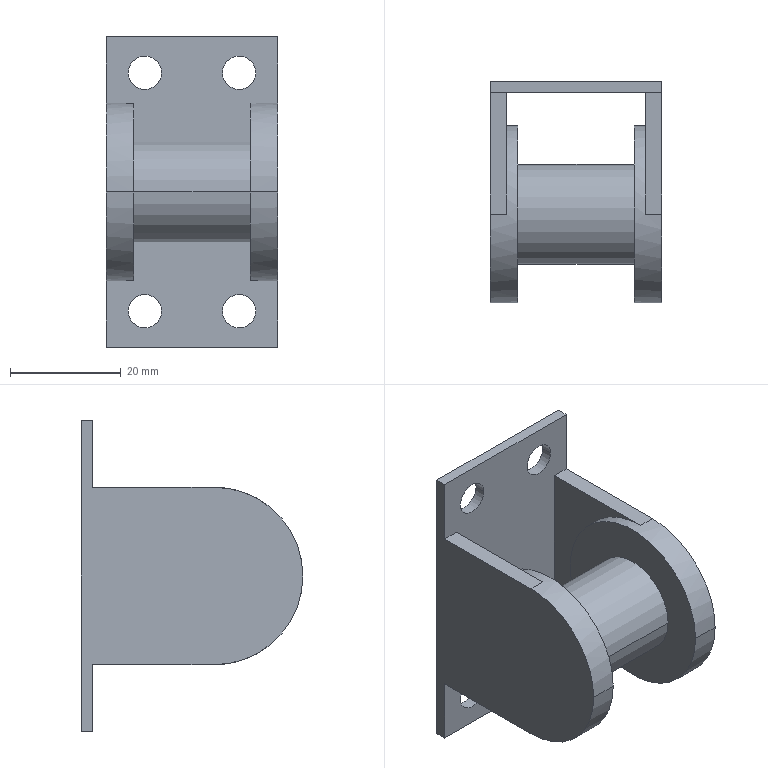Part | SolidWorks | features ICE 3, MirrorPattern 1, Revolution 1 | 1 solid | 28 faces | box 31 x 40 x 56 mm | volume 18443 mm3 | cylinder 14 | plane 14 | commonest cylinder face diameters 6 x8 32 x4 18 x2
STEP:
#1=CARTESIAN_POINT('',(18.,22.,-21.5));
#2=VERTEX_POINT('',#1);
#3=CARTESIAN_POINT('',(24.,22.,-21.5));
#4=VERTEX_POINT('',#3);
#5=CARTESIAN_POINT('',(21.,22.,-21.5));
#6=DIRECTION('',(0.,-1.,0.));
#7=DIRECTION('',(0.,0.,1.));
#8=AXIS2_PLACEMENT_3D('',#5,#6,#7);
#9=CIRCLE('',#8,3.);
#10=EDGE_CURVE('',#2,#4,#9,.T.);
#11=ORIENTED_EDGE('',*,*,#10,.T.);
#12=CARTESIAN_POINT('',(24.,24.,-21.5));
#13=VERTEX_POINT('',#12);
#14=CARTESIAN_POINT('',(24.,-16.001,-21.5));
#15=DIRECTION('',(0.,1.,0.));
#16=VECTOR('',#15,1000.);
#17=LINE('',#14,#16);
#18=EDGE_CURVE('',#4,#13,#17,.T.);
#19=ORIENTED_EDGE('',*,*,#18,.T.);
#20=CARTESIAN_POINT('',(18.,24.,-21.5));
#21=VERTEX_POINT('',#20);
#22=CARTESIAN_POINT('',(21.,24.,-21.5));
#23=DIRECTION('',(0.,1.,0.));
#24=DIRECTION('',(1.,0.,0.));
#25=AXIS2_PLACEMENT_3D('',#22,#23,#24);
#26=CIRCLE('',#25,3.);
#27=EDGE_CURVE('',#13,#21,#26,.T.);
#28=ORIENTED_EDGE('',*,*,#27,.T.);
#29=CARTESIAN_POINT('',(18.,-16.001,-21.5));
#30=DIRECTION('',(0.,1.,0.));
#31=VECTOR('',#30,1000.);
#32=LINE('',#29,#31);
#33=EDGE_CURVE('',#2,#21,#32,.T.);
#34=ORIENTED_EDGE('',*,*,#33,.F.);
#35=EDGE_LOOP('',(#11,#19,#28,#34));
#36=FACE_OUTER_BOUND('',#35,.T.);
#37=CARTESIAN_POINT('',(21.,-16.001,-21.5));
#38=DIRECTION('',(0.,1.,0.));
#39=DIRECTION('',(-1.,0.,0.));
#40=AXIS2_PLACEMENT_3D('',#37,#38,#39);
#41=CYLINDRICAL_SURFACE('',#40,3.);
#42=ADVANCED_FACE('',(#36),#41,.F.);
#43=CARTESIAN_POINT('',(18.,22.,21.5));
#44=VERTEX_POINT('',#43);
#45=CARTESIAN_POINT('',(24.,22.,21.5));
#46=VERTEX_POINT('',#45);
#47=CARTESIAN_POINT('',(21.,22.,21.5));
#48=DIRECTION('',(0.,-1.,0.));
#49=DIRECTION('',(0.,0.,1.));
#50=AXIS2_PLACEMENT_3D('',#47,#48,#49);
#51=CIRCLE('',#50,3.);
#52=EDGE_CURVE('',#44,#46,#51,.T.);
#53=ORIENTED_EDGE('',*,*,#52,.T.);
#54=CARTESIAN_POINT('',(24.,24.,21.5));
#55=VERTEX_POINT('',#54);
#56=CARTESIAN_POINT('',(24.,-16.001,21.5));
#57=DIRECTION('',(0.,1.,0.));
#58=VECTOR('',#57,1000.);
#59=LINE('',#56,#58);
#60=EDGE_CURVE('',#46,#55,#59,.T.);
#61=ORIENTED_EDGE('',*,*,#60,.T.);
#62=CARTESIAN_POINT('',(18.,24.,21.5));
#63=VERTEX_POINT('',#62);
#64=CARTESIAN_POINT('',(21.,24.,21.5));
#65=DIRECTION('',(0.,1.,0.));
#66=DIRECTION('',(-1.,0.,0.));
#67=AXIS2_PLACEMENT_3D('',#64,#65,#66);
#68=CIRCLE('',#67,3.);
#69=EDGE_CURVE('',#55,#63,#68,.T.);
#70=ORIENTED_EDGE('',*,*,#69,.T.);
#71=CARTESIAN_POINT('',(18.,-16.001,21.5));
#72=DIRECTION('',(0.,1.,0.));
#73=VECTOR('',#72,1000.);
#74=LINE('',#71,#73);
#75=EDGE_CURVE('',#44,#63,#74,.T.);
#76=ORIENTED_EDGE('',*,*,#75,.F.);
#77=EDGE_LOOP('',(#53,#61,#70,#76));
#78=FACE_OUTER_BOUND('',#77,.T.);
#79=CARTESIAN_POINT('',(21.,-16.001,21.5));
#80=DIRECTION('',(0.,1.,0.));
#81=DIRECTION('',(-1.,0.,0.));
#82=AXIS2_PLACEMENT_3D('',#79,#80,#81);
#83=CYLINDRICAL_SURFACE('',#82,3.);
#84=ADVANCED_FACE('',(#78),#83,.F.);
#85=CARTESIAN_POINT('',(1.,22.,21.5));
#86=VERTEX_POINT('',#85);
#87=CARTESIAN_POINT('',(7.,22.,21.5));
#88=VERTEX_POINT('',#87);
#89=CARTESIAN_POINT('',(4.,22.,21.5));
#90=DIRECTION('',(0.,-1.,0.));
#91=DIRECTION('',(0.,0.,1.));
#92=AXIS2_PLACEMENT_3D('',#89,#90,#91);
#93=CIRCLE('',#92,3.);
#94=EDGE_CURVE('',#86,#88,#93,.T.);
#95=ORIENTED_EDGE('',*,*,#94,.T.);
#96=CARTESIAN_POINT('',(7.,24.,21.5));
#97=VERTEX_POINT('',#96);
#98=CARTESIAN_POINT('',(7.,-16.001,21.5));
#99=DIRECTION('',(0.,1.,0.));
#100=VECTOR('',#99,1000.);
#101=LINE('',#98,#100);
#102=EDGE_CURVE('',#88,#97,#101,.T.);
#103=ORIENTED_EDGE('',*,*,#102,.T.);
#104=CARTESIAN_POINT('',(1.,24.,21.5));
#105=VERTEX_POINT('',#104);
#106=CARTESIAN_POINT('',(4.,24.,21.5));
#107=DIRECTION('',(0.,1.,0.));
#108=DIRECTION('',(1.,0.,0.));
#109=AXIS2_PLACEMENT_3D('',#106,#107,#108);
#110=CIRCLE('',#109,3.);
#111=EDGE_CURVE('',#97,#105,#110,.T.);
#112=ORIENTED_EDGE('',*,*,#111,.T.);
#113=CARTESIAN_POINT('',(1.,-16.001,21.5));
#114=DIRECTION('',(0.,1.,0.));
#115=VECTOR('',#114,1000.);
#116=LINE('',#113,#115);
#117=EDGE_CURVE('',#86,#105,#116,.T.);
#118=ORIENTED_EDGE('',*,*,#117,.F.);
#119=EDGE_LOOP('',(#95,#103,#112,#118));
#120=FACE_OUTER_BOUND('',#119,.T.);
#121=CARTESIAN_POINT('',(4.,-16.001,21.5));
#122=DIRECTION('',(0.,1.,0.));
#123=DIRECTION('',(-1.,0.,0.));
#124=AXIS2_PLACEMENT_3D('',#121,#122,#123);
#125=CYLINDRICAL_SURFACE('',#124,3.);
#126=ADVANCED_FACE('',(#120),#125,.F.);
#127=CARTESIAN_POINT('',(1.,22.,-21.5));
#128=VERTEX_POINT('',#127);
#129=CARTESIAN_POINT('',(7.,22.,-21.5));
#130=VERTEX_POINT('',#129);
#131=CARTESIAN_POINT('',(4.,22.,-21.5));
#132=DIRECTION('',(0.,-1.,0.));
#133=DIRECTION('',(0.,0.,1.));
#134=AXIS2_PLACEMENT_3D('',#131,#132,#133);
#135=CIRCLE('',#134,3.);
#136=EDGE_CURVE('',#128,#130,#135,.T.);
#137=ORIENTED_EDGE('',*,*,#136,.T.);
#138=CARTESIAN_POINT('',(7.,24.,-21.5));
#139=VERTEX_POINT('',#138);
#140=CARTESIAN_POINT('',(7.,-16.001,-21.5));
#141=DIRECTION('',(0.,1.,0.));
#142=VECTOR('',#141,1000.);
#143=LINE('',#140,#142);
#144=EDGE_CURVE('',#130,#139,#143,.T.);
#145=ORIENTED_EDGE('',*,*,#144,.T.);
#146=CARTESIAN_POINT('',(1.,24.,-21.5));
#147=VERTEX_POINT('',#146);
#148=CARTESIAN_POINT('',(4.,24.,-21.5));
#149=DIRECTION('',(0.,1.,0.));
#150=DIRECTION('',(-1.,0.,0.));
#151=AXIS2_PLACEMENT_3D('',#148,#149,#150);
#152=CIRCLE('',#151,3.);
#153=EDGE_CURVE('',#139,#147,#152,.T.);
#154=ORIENTED_EDGE('',*,*,#153,.T.);
#155=CARTESIAN_POINT('',(1.,-16.001,-21.5));
#156=DIRECTION('',(0.,1.,0.));
#157=VECTOR('',#156,1000.);
#158=LINE('',#155,#157);
#159=EDGE_CURVE('',#128,#147,#158,.T.);
#160=ORIENTED_EDGE('',*,*,#159,.F.);
#161=EDGE_LOOP('',(#137,#145,#154,#160));
#162=FACE_OUTER_BOUND('',#161,.T.);
#163=CARTESIAN_POINT('',(4.,-16.001,-21.5));
#164=DIRECTION('',(0.,1.,0.));
#165=DIRECTION('',(-1.,0.,0.));
#166=AXIS2_PLACEMENT_3D('',#163,#164,#165);
#167=CYLINDRICAL_SURFACE('',#166,3.);
#168=ADVANCED_FACE('',(#162),#167,.F.);
#169=CARTESIAN_POINT('',(2.,9.,0.));
#170=VERTEX_POINT('',#169);
#171=CARTESIAN_POINT('',(2.,-9.,0.));
#172=VERTEX_POINT('',#171);
#173=CARTESIAN_POINT('',(2.,0.,0.));
#174=DIRECTION('',(1.,0.,0.));
#175=DIRECTION('',(0.,1.,0.));
#176=AXIS2_PLACEMENT_3D('',#173,#174,#175);
#177=CIRCLE('',#176,9.);
#178=EDGE_CURVE('',#170,#172,#177,.T.);
#179=ORIENTED_EDGE('',*,*,#178,.T.);
#180=CARTESIAN_POINT('',(23.,-9.,0.));
#181=VERTEX_POINT('',#180);
#182=CARTESIAN_POINT('',(25.,-9.,0.));
#183=DIRECTION('',(1.,0.,0.));
#184=VECTOR('',#183,1000.);
#185=LINE('',#182,#184);
#186=EDGE_CURVE('',#172,#181,#185,.T.);
#187=ORIENTED_EDGE('',*,*,#186,.T.);
#188=CARTESIAN_POINT('',(23.,9.,0.));
#189=VERTEX_POINT('',#188);
#190=CARTESIAN_POINT('',(23.,0.,0.));
#191=DIRECTION('',(1.,0.,0.));
#192=DIRECTION('',(0.,1.,0.));
#193=AXIS2_PLACEMENT_3D('',#190,#191,#192);
#194=CIRCLE('',#193,9.);
#195=EDGE_CURVE('',#189,#181,#194,.T.);
#196=ORIENTED_EDGE('',*,*,#195,.F.);
#197=CARTESIAN_POINT('',(25.,9.,0.));
#198=DIRECTION('',(1.,0.,0.));
#199=VECTOR('',#198,1000.);
#200=LINE('',#197,#199);
#201=EDGE_CURVE('',#170,#189,#200,.T.);
#202=ORIENTED_EDGE('',*,*,#201,.F.);
#203=EDGE_LOOP('',(#179,#187,#196,#202));
#204=FACE_OUTER_BOUND('',#203,.T.);
#205=CARTESIAN_POINT('',(25.,0.,0.));
#206=DIRECTION('',(1.,0.,0.));
#207=DIRECTION('',(0.,1.,0.));
#208=AXIS2_PLACEMENT_3D('',#205,#206,#207);
#209=CYLINDRICAL_SURFACE('',#208,9.);
#210=ADVANCED_FACE('',(#204),#209,.T.);
#211=CARTESIAN_POINT('',(23.,16.,0.));
#212=VERTEX_POINT('',#211);
#213=CARTESIAN_POINT('',(23.,-16.,0.));
#214=VERTEX_POINT('',#213);
#215=CARTESIAN_POINT('',(23.,0.,0.));
#216=DIRECTION('',(1.,0.,0.));
#217=DIRECTION('',(0.,1.,0.));
#218=AXIS2_PLACEMENT_3D('',#215,#216,#217);
#219=CIRCLE('',#218,16.);
#220=EDGE_CURVE('',#212,#214,#219,.T.);
#221=ORIENTED_EDGE('',*,*,#220,.T.);
#222=CARTESIAN_POINT('',(28.,-16.,0.));
#223=VERTEX_POINT('',#222);
#224=CARTESIAN_POINT('',(25.,-16.,0.));
#225=DIRECTION('',(1.,0.,0.));
#226=VECTOR('',#225,1000.);
#227=LINE('',#224,#226);
#228=EDGE_CURVE('',#214,#223,#227,.T.);
#229=ORIENTED_EDGE('',*,*,#228,.T.);
#230=CARTESIAN_POINT('',(28.,0.,16.));
#231=VERTEX_POINT('',#230);
#232=CARTESIAN_POINT('',(28.,0.,0.));
#233=DIRECTION('',(-1.,0.,0.));
#234=DIRECTION('',(0.,-1.,0.));
#235=AXIS2_PLACEMENT_3D('',#232,#233,#234);
#236=CIRCLE('',#235,16.);
#237=EDGE_CURVE('',#223,#231,#236,.T.);
#238=ORIENTED_EDGE('',*,*,#237,.T.);
#239=CARTESIAN_POINT('',(25.,0.,16.));
#240=VERTEX_POINT('',#239);
#241=CARTESIAN_POINT('',(28.,0.,16.));
#242=DIRECTION('',(-1.,0.,0.));
#243=VECTOR('',#242,1000.);
#244=LINE('',#241,#243);
#245=EDGE_CURVE('',#231,#240,#244,.T.);
#246=ORIENTED_EDGE('',*,*,#245,.T.);
#247=CARTESIAN_POINT('',(25.,16.,0.));
#248=VERTEX_POINT('',#247);
#249=CARTESIAN_POINT('',(25.,0.,0.));
#250=DIRECTION('',(1.,0.,0.));
#251=DIRECTION('',(0.,1.,0.));
#252=AXIS2_PLACEMENT_3D('',#249,#250,#251);
#253=CIRCLE('',#252,16.);
#254=EDGE_CURVE('',#248,#240,#253,.T.);
#255=ORIENTED_EDGE('',*,*,#254,.F.);
#256=CARTESIAN_POINT('',(25.,16.,0.));
#257=DIRECTION('',(1.,0.,0.));
#258=VECTOR('',#257,1000.);
#259=LINE('',#256,#258);
#260=EDGE_CURVE('',#212,#248,#259,.T.);
#261=ORIENTED_EDGE('',*,*,#260,.F.);
#262=EDGE_LOOP('',(#221,#229,#238,#246,#255,#261));
#263=FACE_OUTER_BOUND('',#262,.T.);
#264=CARTESIAN_POINT('',(25.,0.,0.));
#265=DIRECTION('',(1.,0.,0.));
#266=DIRECTION('',(0.,1.,0.));
#267=AXIS2_PLACEMENT_3D('',#264,#265,#266);
#268=CYLINDRICAL_SURFACE('',#267,16.);
#269=ADVANCED_FACE('',(#263),#268,.T.);
#270=CARTESIAN_POINT('',(-3.,-16.,0.));
#271=VERTEX_POINT('',#270);
#272=CARTESIAN_POINT('',(-3.,0.,16.));
#273=VERTEX_POINT('',#272);
#274=CARTESIAN_POINT('',(-3.,0.,0.));
#275=DIRECTION('',(-1.,0.,0.));
#276=DIRECTION('',(0.,-1.,0.));
#277=AXIS2_PLACEMENT_3D('',#274,#275,#276);
#278=CIRCLE('',#277,16.);
#279=EDGE_CURVE('',#271,#273,#278,.T.);
#280=ORIENTED_EDGE('',*,*,#279,.F.);
#281=CARTESIAN_POINT('',(2.,-16.,0.));
#282=VERTEX_POINT('',#281);
#283=CARTESIAN_POINT('',(25.,-16.,0.));
#284=DIRECTION('',(1.,0.,0.));
#285=VECTOR('',#284,1000.);
#286=LINE('',#283,#285);
#287=EDGE_CURVE('',#271,#282,#286,.T.);
#288=ORIENTED_EDGE('',*,*,#287,.T.);
#289=CARTESIAN_POINT('',(2.,16.,0.));
#290=VERTEX_POINT('',#289);
#291=CARTESIAN_POINT('',(2.,0.,0.));
#292=DIRECTION('',(1.,0.,0.));
#293=DIRECTION('',(0.,1.,0.));
#294=AXIS2_PLACEMENT_3D('',#291,#292,#293);
#295=CIRCLE('',#294,16.);
#296=EDGE_CURVE('',#290,#282,#295,.T.);
#297=ORIENTED_EDGE('',*,*,#296,.F.);
#298=CARTESIAN_POINT('',(0.,16.,0.));
#299=VERTEX_POINT('',#298);
#300=CARTESIAN_POINT('',(25.,16.,0.));
#301=DIRECTION('',(1.,0.,0.));
#302=VECTOR('',#301,1000.);
#303=LINE('',#300,#302);
#304=EDGE_CURVE('',#299,#290,#303,.T.);
#305=ORIENTED_EDGE('',*,*,#304,.F.);
#306=CARTESIAN_POINT('',(0.,0.,16.));
#307=VERTEX_POINT('',#306);
#308=CARTESIAN_POINT('',(0.,0.,0.));
#309=DIRECTION('',(1.,0.,0.));
#310=DIRECTION('',(0.,1.,0.));
#311=AXIS2_PLACEMENT_3D('',#308,#309,#310);
#312=CIRCLE('',#311,16.);
#313=EDGE_CURVE('',#299,#307,#312,.T.);
#314=ORIENTED_EDGE('',*,*,#313,.T.);
#315=CARTESIAN_POINT('',(-3.,0.,16.));
#316=DIRECTION('',(1.,0.,0.));
#317=VECTOR('',#316,1000.);
#318=LINE('',#315,#317);
#319=EDGE_CURVE('',#273,#307,#318,.T.);
#320=ORIENTED_EDGE('',*,*,#319,.F.);
#321=EDGE_LOOP('',(#280,#288,#297,#305,#314,#320));
#322=FACE_OUTER_BOUND('',#321,.T.);
#323=CARTESIAN_POINT('',(25.,0.,0.));
#324=DIRECTION('',(1.,0.,0.));
#325=DIRECTION('',(0.,1.,0.));
#326=AXIS2_PLACEMENT_3D('',#323,#324,#325);
#327=CYLINDRICAL_SURFACE('',#326,16.);
#328=ADVANCED_FACE('',(#322),#327,.T.);
#329=CARTESIAN_POINT('',(-3.,22.,16.));
#330=VERTEX_POINT('',#329);
#331=CARTESIAN_POINT('',(0.,22.,16.));
#332=VERTEX_POINT('',#331);
#333=CARTESIAN_POINT('',(-3.,22.,16.));
#334=DIRECTION('',(1.,0.,0.));
#335=VECTOR('',#334,1000.);
#336=LINE('',#333,#335);
#337=EDGE_CURVE('',#330,#332,#336,.T.);
#338=ORIENTED_EDGE('',*,*,#337,.F.);
#339=CARTESIAN_POINT('',(-3.,0.,16.));
#340=DIRECTION('',(0.,1.,0.));
#341=VECTOR('',#340,1000.);
#342=LINE('',#339,#341);
#343=EDGE_CURVE('',#273,#330,#342,.T.);
#344=ORIENTED_EDGE('',*,*,#343,.F.);
#345=ORIENTED_EDGE('',*,*,#319,.T.);
#346=CARTESIAN_POINT('',(0.,0.,16.));
#347=DIRECTION('',(0.,1.,0.));
#348=VECTOR('',#347,1000.);
#349=LINE('',#346,#348);
#350=EDGE_CURVE('',#307,#332,#349,.T.);
#351=ORIENTED_EDGE('',*,*,#350,.T.);
#352=EDGE_LOOP('',(#338,#344,#345,#351));
#353=FACE_OUTER_BOUND('',#352,.T.);
#354=CARTESIAN_POINT('',(-3.,0.,16.));
#355=DIRECTION('',(0.,0.,-1.));
#356=DIRECTION('',(-1.,0.,0.));
#357=AXIS2_PLACEMENT_3D('',#354,#355,#356);
#358=PLANE('',#357);
#359=ADVANCED_FACE('',(#353),#358,.F.);
#360=CARTESIAN_POINT('',(0.,22.,-16.));
#361=VERTEX_POINT('',#360);
#362=CARTESIAN_POINT('',(-3.,22.,-16.));
#363=VERTEX_POINT('',#362);
#364=CARTESIAN_POINT('',(-3.,22.,-16.));
#365=DIRECTION('',(-1.,0.,0.));
#366=VECTOR('',#365,1000.);
#367=LINE('',#364,#366);
#368=EDGE_CURVE('',#361,#363,#367,.T.);
#369=ORIENTED_EDGE('',*,*,#368,.F.);
#370=CARTESIAN_POINT('',(0.,0.,-16.));
#371=VERTEX_POINT('',#370);
#372=CARTESIAN_POINT('',(0.,0.,-16.));
#373=DIRECTION('',(0.,-1.,0.));
#374=VECTOR('',#373,1000.);
#375=LINE('',#372,#374);
#376=EDGE_CURVE('',#361,#371,#375,.T.);
#377=ORIENTED_EDGE('',*,*,#376,.T.);
#378=CARTESIAN_POINT('',(-3.,0.,-16.));
#379=VERTEX_POINT('',#378);
#380=CARTESIAN_POINT('',(-3.,0.,-16.));
#381=DIRECTION('',(1.,0.,0.));
#382=VECTOR('',#381,1000.);
#383=LINE('',#380,#382);
#384=EDGE_CURVE('',#379,#371,#383,.T.);
#385=ORIENTED_EDGE('',*,*,#384,.F.);
#386=CARTESIAN_POINT('',(-3.,0.,-16.));
#387=DIRECTION('',(0.,-1.,0.));
#388=VECTOR('',#387,1000.);
#389=LINE('',#386,#388);
#390=EDGE_CURVE('',#363,#379,#389,.T.);
#391=ORIENTED_EDGE('',*,*,#390,.F.);
#392=EDGE_LOOP('',(#369,#377,#385,#391));
#393=FACE_OUTER_BOUND('',#392,.T.);
#394=CARTESIAN_POINT('',(-3.,0.,-16.));
#395=DIRECTION('',(0.,0.,1.));
#396=DIRECTION('',(0.,-1.,0.));
#397=AXIS2_PLACEMENT_3D('',#394,#395,#396);
#398=PLANE('',#397);
#399=ADVANCED_FACE('',(#393),#398,.F.);
#400=CARTESIAN_POINT('',(0.,22.,0.));
#401=DIRECTION('',(0.,0.,-1.));
#402=VECTOR('',#401,1000.);
#403=LINE('',#400,#402);
#404=EDGE_CURVE('',#332,#361,#403,.T.);
#405=ORIENTED_EDGE('',*,*,#404,.F.);
#406=ORIENTED_EDGE('',*,*,#350,.F.);
#407=ORIENTED_EDGE('',*,*,#313,.F.);
#408=CARTESIAN_POINT('',(0.,0.,0.));
#409=DIRECTION('',(1.,0.,0.));
#410=DIRECTION('',(0.,1.,0.));
#411=AXIS2_PLACEMENT_3D('',#408,#409,#410);
#412=CIRCLE('',#411,16.);
#413=EDGE_CURVE('',#371,#299,#412,.T.);
#414=ORIENTED_EDGE('',*,*,#413,.F.);
#415=ORIENTED_EDGE('',*,*,#376,.F.);
#416=EDGE_LOOP('',(#405,#406,#407,#414,#415));
#417=FACE_OUTER_BOUND('',#416,.T.);
#418=CARTESIAN_POINT('',(0.,0.,0.));
#419=DIRECTION('',(-1.,0.,0.));
#420=DIRECTION('',(0.,-1.,0.));
#421=AXIS2_PLACEMENT_3D('',#418,#419,#420);
#422=PLANE('',#421);
#423=ADVANCED_FACE('',(#417),#422,.F.);
#424=CARTESIAN_POINT('',(25.,22.,-16.));
#425=VERTEX_POINT('',#424);
#426=CARTESIAN_POINT('',(25.,22.,16.));
#427=VERTEX_POINT('',#426);
#428=CARTESIAN_POINT('',(25.,22.,0.));
#429=DIRECTION('',(0.,0.,1.));
#430=VECTOR('',#429,1000.);
#431=LINE('',#428,#430);
#432=EDGE_CURVE('',#425,#427,#431,.T.);
#433=ORIENTED_EDGE('',*,*,#432,.F.);
#434=CARTESIAN_POINT('',(25.,0.,-16.));
#435=VERTEX_POINT('',#434);
#436=CARTESIAN_POINT('',(25.,0.,-16.));
#437=DIRECTION('',(0.,-1.,0.));
#438=VECTOR('',#437,1000.);
#439=LINE('',#436,#438);
#440=EDGE_CURVE('',#425,#435,#439,.T.);
#441=ORIENTED_EDGE('',*,*,#440,.T.);
#442=CARTESIAN_POINT('',(25.,0.,0.));
#443=DIRECTION('',(1.,0.,0.));
#444=DIRECTION('',(0.,1.,0.));
#445=AXIS2_PLACEMENT_3D('',#442,#443,#444);
#446=CIRCLE('',#445,16.);
#447=EDGE_CURVE('',#435,#248,#446,.T.);
#448=ORIENTED_EDGE('',*,*,#447,.T.);
#449=ORIENTED_EDGE('',*,*,#254,.T.);
#450=CARTESIAN_POINT('',(25.,0.,16.));
#451=DIRECTION('',(0.,1.,0.));
#452=VECTOR('',#451,1000.);
#453=LINE('',#450,#452);
#454=EDGE_CURVE('',#240,#427,#453,.T.);
#455=ORIENTED_EDGE('',*,*,#454,.T.);
#456=EDGE_LOOP('',(#433,#441,#448,#449,#455));
#457=FACE_OUTER_BOUND('',#456,.T.);
#458=CARTESIAN_POINT('',(25.,0.,0.));
#459=DIRECTION('',(1.,0.,0.));
#460=DIRECTION('',(0.,-1.,0.));
#461=AXIS2_PLACEMENT_3D('',#458,#459,#460);
#462=PLANE('',#461);
#463=ADVANCED_FACE('',(#457),#462,.F.);
#464=CARTESIAN_POINT('',(28.,22.,16.));
#465=VERTEX_POINT('',#464);
#466=CARTESIAN_POINT('',(28.,0.,16.));
#467=DIRECTION('',(0.,1.,0.));
#468=VECTOR('',#467,1000.);
#469=LINE('',#466,#468);
#470=EDGE_CURVE('',#231,#465,#469,.T.);
#471=ORIENTED_EDGE('',*,*,#470,.T.);
#472=CARTESIAN_POINT('',(28.,22.,16.));
#473=DIRECTION('',(-1.,0.,0.));
#474=VECTOR('',#473,1000.);
#475=LINE('',#472,#474);
#476=EDGE_CURVE('',#465,#427,#475,.T.);
#477=ORIENTED_EDGE('',*,*,#476,.T.);
#478=ORIENTED_EDGE('',*,*,#454,.F.);
#479=ORIENTED_EDGE('',*,*,#245,.F.);
#480=EDGE_LOOP('',(#471,#477,#478,#479));
#481=FACE_OUTER_BOUND('',#480,.T.);
#482=CARTESIAN_POINT('',(28.,0.,16.));
#483=DIRECTION('',(0.,0.,1.));
#484=DIRECTION('',(1.,0.,0.));
#485=AXIS2_PLACEMENT_3D('',#482,#483,#484);
#486=PLANE('',#485);
#487=ADVANCED_FACE('',(#481),#486,.T.);
#488=ORIENTED_EDGE('',*,*,#440,.F.);
#489=CARTESIAN_POINT('',(28.,22.,-16.));
#490=VERTEX_POINT('',#489);
#491=CARTESIAN_POINT('',(28.,22.,-16.));
#492=DIRECTION('',(1.,0.,0.));
#493=VECTOR('',#492,1000.);
#494=LINE('',#491,#493);
#495=EDGE_CURVE('',#425,#490,#494,.T.);
#496=ORIENTED_EDGE('',*,*,#495,.T.);
#497=CARTESIAN_POINT('',(28.,0.,-16.));
#498=VERTEX_POINT('',#497);
#499=CARTESIAN_POINT('',(28.,0.,-16.));
#500=DIRECTION('',(0.,-1.,0.));
#501=VECTOR('',#500,1000.);
#502=LINE('',#499,#501);
#503=EDGE_CURVE('',#490,#498,#502,.T.);
#504=ORIENTED_EDGE('',*,*,#503,.T.);
#505=CARTESIAN_POINT('',(28.,0.,-16.));
#506=DIRECTION('',(-1.,0.,0.));
#507=VECTOR('',#506,1000.);
#508=LINE('',#505,#507);
#509=EDGE_CURVE('',#498,#435,#508,.T.);
#510=ORIENTED_EDGE('',*,*,#509,.T.);
#511=EDGE_LOOP('',(#488,#496,#504,#510));
#512=FACE_OUTER_BOUND('',#511,.T.);
#513=CARTESIAN_POINT('',(28.,0.,-16.));
#514=DIRECTION('',(0.,0.,-1.));
#515=DIRECTION('',(0.,1.,0.));
#516=AXIS2_PLACEMENT_3D('',#513,#514,#515);
#517=PLANE('',#516);
#518=ADVANCED_FACE('',(#512),#517,.T.);
#519=ORIENTED_EDGE('',*,*,#287,.F.);
#520=CARTESIAN_POINT('',(-3.,0.,0.));
#521=DIRECTION('',(-1.,0.,0.));
#522=DIRECTION('',(0.,-1.,0.));
#523=AXIS2_PLACEMENT_3D('',#520,#521,#522);
#524=CIRCLE('',#523,16.);
#525=EDGE_CURVE('',#379,#271,#524,.T.);
#526=ORIENTED_EDGE('',*,*,#525,.F.);
#527=ORIENTED_EDGE('',*,*,#384,.T.);
#528=ORIENTED_EDGE('',*,*,#413,.T.);
#529=ORIENTED_EDGE('',*,*,#304,.T.);
#530=CARTESIAN_POINT('',(2.,0.,0.));
#531=DIRECTION('',(1.,0.,0.));
#532=DIRECTION('',(0.,1.,0.));
#533=AXIS2_PLACEMENT_3D('',#530,#531,#532);
#534=CIRCLE('',#533,16.);
#535=EDGE_CURVE('',#282,#290,#534,.T.);
#536=ORIENTED_EDGE('',*,*,#535,.F.);
#537=EDGE_LOOP('',(#519,#526,#527,#528,#529,#536));
#538=FACE_OUTER_BOUND('',#537,.T.);
#539=CARTESIAN_POINT('',(25.,0.,0.));
#540=DIRECTION('',(1.,0.,0.));
#541=DIRECTION('',(0.,1.,0.));
#542=AXIS2_PLACEMENT_3D('',#539,#540,#541);
#543=CYLINDRICAL_SURFACE('',#542,16.);
#544=ADVANCED_FACE('',(#538),#543,.T.);
#545=ORIENTED_EDGE('',*,*,#228,.F.);
#546=CARTESIAN_POINT('',(23.,0.,0.));
#547=DIRECTION('',(1.,0.,0.));
#548=DIRECTION('',(0.,1.,0.));
#549=AXIS2_PLACEMENT_3D('',#546,#547,#548);
#550=CIRCLE('',#549,16.);
#551=EDGE_CURVE('',#214,#212,#550,.T.);
#552=ORIENTED_EDGE('',*,*,#551,.T.);
#553=ORIENTED_EDGE('',*,*,#260,.T.);
#554=ORIENTED_EDGE('',*,*,#447,.F.);
#555=ORIENTED_EDGE('',*,*,#509,.F.);
#556=CARTESIAN_POINT('',(28.,0.,0.));
#557=DIRECTION('',(-1.,0.,0.));
#558=DIRECTION('',(0.,-1.,0.));
#559=AXIS2_PLACEMENT_3D('',#556,#557,#558);
#560=CIRCLE('',#559,16.);
#561=EDGE_CURVE('',#498,#223,#560,.T.);
#562=ORIENTED_EDGE('',*,*,#561,.T.);
#563=EDGE_LOOP('',(#545,#552,#553,#554,#555,#562));
#564=FACE_OUTER_BOUND('',#563,.T.);
#565=CARTESIAN_POINT('',(25.,0.,0.));
#566=DIRECTION('',(1.,0.,0.));
#567=DIRECTION('',(0.,1.,0.));
#568=AXIS2_PLACEMENT_3D('',#565,#566,#567);
#569=CYLINDRICAL_SURFACE('',#568,16.);
#570=ADVANCED_FACE('',(#564),#569,.T.);
#571=ORIENTED_EDGE('',*,*,#220,.F.);
#572=ORIENTED_EDGE('',*,*,#551,.F.);
#573=EDGE_LOOP('',(#571,#572));
#574=FACE_OUTER_BOUND('',#573,.T.);
#575=ORIENTED_EDGE('',*,*,#195,.T.);
#576=CARTESIAN_POINT('',(23.,0.,0.));
#577=DIRECTION('',(1.,0.,0.));
#578=DIRECTION('',(0.,1.,0.));
#579=AXIS2_PLACEMENT_3D('',#576,#577,#578);
#580=CIRCLE('',#579,9.);
#581=EDGE_CURVE('',#181,#189,#580,.T.);
#582=ORIENTED_EDGE('',*,*,#581,.T.);
#583=EDGE_LOOP('',(#575,#582));
#584=FACE_BOUND('',#583,.T.);
#585=CARTESIAN_POINT('',(23.,0.,0.));
#586=DIRECTION('',(1.,0.,0.));
#587=DIRECTION('',(0.,1.,0.));
#588=AXIS2_PLACEMENT_3D('',#585,#586,#587);
#589=PLANE('',#588);
#590=ADVANCED_FACE('',(#574,#584),#589,.F.);
#591=ORIENTED_EDGE('',*,*,#186,.F.);
#592=CARTESIAN_POINT('',(2.,0.,0.));
#593=DIRECTION('',(1.,0.,0.));
#594=DIRECTION('',(0.,1.,0.));
#595=AXIS2_PLACEMENT_3D('',#592,#593,#594);
#596=CIRCLE('',#595,9.);
#597=EDGE_CURVE('',#172,#170,#596,.T.);
#598=ORIENTED_EDGE('',*,*,#597,.T.);
#599=ORIENTED_EDGE('',*,*,#201,.T.);
#600=ORIENTED_EDGE('',*,*,#581,.F.);
#601=EDGE_LOOP('',(#591,#598,#599,#600));
#602=FACE_OUTER_BOUND('',#601,.T.);
#603=CARTESIAN_POINT('',(25.,0.,0.));
#604=DIRECTION('',(1.,0.,0.));
#605=DIRECTION('',(0.,1.,0.));
#606=AXIS2_PLACEMENT_3D('',#603,#604,#605);
#607=CYLINDRICAL_SURFACE('',#606,9.);
#608=ADVANCED_FACE('',(#602),#607,.T.);
#609=ORIENTED_EDGE('',*,*,#178,.F.);
#610=ORIENTED_EDGE('',*,*,#597,.F.);
#611=EDGE_LOOP('',(#609,#610));
#612=FACE_BOUND('',#611,.T.);
#613=ORIENTED_EDGE('',*,*,#296,.T.);
#614=ORIENTED_EDGE('',*,*,#535,.T.);
#615=EDGE_LOOP('',(#613,#614));
#616=FACE_OUTER_BOUND('',#615,.T.);
#617=CARTESIAN_POINT('',(2.,0.,0.));
#618=DIRECTION('',(-1.,0.,0.));
#619=DIRECTION('',(0.,-1.,0.));
#620=AXIS2_PLACEMENT_3D('',#617,#618,#619);
#621=PLANE('',#620);
#622=ADVANCED_FACE('',(#612,#616),#621,.F.);
#623=CARTESIAN_POINT('',(21.,24.,-21.5));
#624=DIRECTION('',(0.,1.,0.));
#625=DIRECTION('',(1.,0.,0.));
#626=AXIS2_PLACEMENT_3D('',#623,#624,#625);
#627=CIRCLE('',#626,3.);
#628=EDGE_CURVE('',#21,#13,#627,.T.);
#629=ORIENTED_EDGE('',*,*,#628,.F.);
#630=ORIENTED_EDGE('',*,*,#27,.F.);
#631=EDGE_LOOP('',(#629,#630));
#632=FACE_BOUND('',#631,.T.);
#633=CARTESIAN_POINT('',(21.,24.,21.5));
#634=DIRECTION('',(0.,1.,0.));
#635=DIRECTION('',(-1.,0.,0.));
#636=AXIS2_PLACEMENT_3D('',#633,#634,#635);
#637=CIRCLE('',#636,3.);
#638=EDGE_CURVE('',#63,#55,#637,.T.);
#639=ORIENTED_EDGE('',*,*,#638,.F.);
#640=ORIENTED_EDGE('',*,*,#69,.F.);
#641=EDGE_LOOP('',(#639,#640));
#642=FACE_BOUND('',#641,.T.);
#643=CARTESIAN_POINT('',(4.,24.,21.5));
#644=DIRECTION('',(0.,1.,0.));
#645=DIRECTION('',(1.,0.,0.));
#646=AXIS2_PLACEMENT_3D('',#643,#644,#645);
#647=CIRCLE('',#646,3.);
#648=EDGE_CURVE('',#105,#97,#647,.T.);
#649=ORIENTED_EDGE('',*,*,#648,.F.);
#650=ORIENTED_EDGE('',*,*,#111,.F.);
#651=EDGE_LOOP('',(#649,#650));
#652=FACE_BOUND('',#651,.T.);
#653=CARTESIAN_POINT('',(4.,24.,-21.5));
#654=DIRECTION('',(0.,1.,0.));
#655=DIRECTION('',(-1.,0.,0.));
#656=AXIS2_PLACEMENT_3D('',#653,#654,#655);
#657=CIRCLE('',#656,3.);
#658=EDGE_CURVE('',#147,#139,#657,.T.);
#659=ORIENTED_EDGE('',*,*,#658,.F.);
#660=ORIENTED_EDGE('',*,*,#153,.F.);
#661=EDGE_LOOP('',(#659,#660));
#662=FACE_BOUND('',#661,.T.);
#663=CARTESIAN_POINT('',(-3.,24.,28.));
#664=VERTEX_POINT('',#663);
#665=CARTESIAN_POINT('',(-3.,24.,-28.));
#666=VERTEX_POINT('',#665);
#667=CARTESIAN_POINT('',(-3.,24.,-16.));
#668=DIRECTION('',(0.,0.,-1.));
#669=VECTOR('',#668,1000.);
#670=LINE('',#667,#669);
#671=EDGE_CURVE('',#664,#666,#670,.T.);
#672=ORIENTED_EDGE('',*,*,#671,.F.);
#673=CARTESIAN_POINT('',(28.,24.,28.));
#674=VERTEX_POINT('',#673);
#675=CARTESIAN_POINT('',(-3.,24.,28.));
#676=DIRECTION('',(-1.,0.,0.));
#677=VECTOR('',#676,1000.);
#678=LINE('',#675,#677);
#679=EDGE_CURVE('',#674,#664,#678,.T.);
#680=ORIENTED_EDGE('',*,*,#679,.F.);
#681=CARTESIAN_POINT('',(28.,24.,-28.));
#682=VERTEX_POINT('',#681);
#683=CARTESIAN_POINT('',(28.,24.,-16.));
#684=DIRECTION('',(0.,0.,-1.));
#685=VECTOR('',#684,1000.);
#686=LINE('',#683,#685);
#687=EDGE_CURVE('',#674,#682,#686,.T.);
#688=ORIENTED_EDGE('',*,*,#687,.T.);
#689=CARTESIAN_POINT('',(-3.,24.,-28.));
#690=DIRECTION('',(-1.,0.,0.));
#691=VECTOR('',#690,1000.);
#692=LINE('',#689,#691);
#693=EDGE_CURVE('',#682,#666,#692,.T.);
#694=ORIENTED_EDGE('',*,*,#693,.T.);
#695=EDGE_LOOP('',(#672,#680,#688,#694));
#696=FACE_OUTER_BOUND('',#695,.T.);
#697=CARTESIAN_POINT('',(-3.,24.,-16.));
#698=DIRECTION('',(0.,-1.,0.));
#699=DIRECTION('',(1.,0.,0.));
#700=AXIS2_PLACEMENT_3D('',#697,#698,#699);
#701=PLANE('',#700);
#702=ADVANCED_FACE('',(#632,#642,#652,#662,#696),#701,.F.);
#703=ORIENTED_EDGE('',*,*,#671,.T.);
#704=CARTESIAN_POINT('',(-3.,22.,-28.));
#705=VERTEX_POINT('',#704);
#706=CARTESIAN_POINT('',(-3.,24.,-28.));
#707=DIRECTION('',(0.,-1.,0.));
#708=VECTOR('',#707,1000.);
#709=LINE('',#706,#708);
#710=EDGE_CURVE('',#666,#705,#709,.T.);
#711=ORIENTED_EDGE('',*,*,#710,.T.);
#712=CARTESIAN_POINT('',(-3.,22.,28.));
#713=DIRECTION('',(0.,0.,-1.));
#714=VECTOR('',#713,1000.);
#715=LINE('',#712,#714);
#716=EDGE_CURVE('',#363,#705,#715,.T.);
#717=ORIENTED_EDGE('',*,*,#716,.F.);
#718=ORIENTED_EDGE('',*,*,#390,.T.);
#719=ORIENTED_EDGE('',*,*,#525,.T.);
#720=ORIENTED_EDGE('',*,*,#279,.T.);
#721=ORIENTED_EDGE('',*,*,#343,.T.);
#722=CARTESIAN_POINT('',(-3.,22.,28.));
#723=VERTEX_POINT('',#722);
#724=CARTESIAN_POINT('',(-3.,22.,28.));
#725=DIRECTION('',(0.,0.,-1.));
#726=VECTOR('',#725,1000.);
#727=LINE('',#724,#726);
#728=EDGE_CURVE('',#723,#330,#727,.T.);
#729=ORIENTED_EDGE('',*,*,#728,.F.);
#730=CARTESIAN_POINT('',(-3.,24.,28.));
#731=DIRECTION('',(0.,-1.,0.));
#732=VECTOR('',#731,1000.);
#733=LINE('',#730,#732);
#734=EDGE_CURVE('',#664,#723,#733,.T.);
#735=ORIENTED_EDGE('',*,*,#734,.F.);
#736=EDGE_LOOP('',(#703,#711,#717,#718,#719,#720,#721,#729,#735));
#737=FACE_OUTER_BOUND('',#736,.T.);
#738=CARTESIAN_POINT('',(-3.,0.,0.));
#739=DIRECTION('',(-1.,0.,0.));
#740=DIRECTION('',(0.,-1.,0.));
#741=AXIS2_PLACEMENT_3D('',#738,#739,#740);
#742=PLANE('',#741);
#743=ADVANCED_FACE('',(#737),#742,.T.);
#744=ORIENTED_EDGE('',*,*,#687,.F.);
#745=CARTESIAN_POINT('',(28.,22.,28.));
#746=VERTEX_POINT('',#745);
#747=CARTESIAN_POINT('',(28.,24.,28.));
#748=DIRECTION('',(0.,1.,0.));
#749=VECTOR('',#748,1000.);
#750=LINE('',#747,#749);
#751=EDGE_CURVE('',#746,#674,#750,.T.);
#752=ORIENTED_EDGE('',*,*,#751,.F.);
#753=CARTESIAN_POINT('',(28.,22.,28.));
#754=DIRECTION('',(0.,0.,-1.));
#755=VECTOR('',#754,1000.);
#756=LINE('',#753,#755);
#757=EDGE_CURVE('',#746,#465,#756,.T.);
#758=ORIENTED_EDGE('',*,*,#757,.T.);
#759=ORIENTED_EDGE('',*,*,#470,.F.);
#760=ORIENTED_EDGE('',*,*,#237,.F.);
#761=ORIENTED_EDGE('',*,*,#561,.F.);
#762=ORIENTED_EDGE('',*,*,#503,.F.);
#763=CARTESIAN_POINT('',(28.,22.,-28.));
#764=VERTEX_POINT('',#763);
#765=CARTESIAN_POINT('',(28.,22.,28.));
#766=DIRECTION('',(0.,0.,-1.));
#767=VECTOR('',#766,1000.);
#768=LINE('',#765,#767);
#769=EDGE_CURVE('',#490,#764,#768,.T.);
#770=ORIENTED_EDGE('',*,*,#769,.T.);
#771=CARTESIAN_POINT('',(28.,24.,-28.));
#772=DIRECTION('',(0.,1.,0.));
#773=VECTOR('',#772,1000.);
#774=LINE('',#771,#773);
#775=EDGE_CURVE('',#764,#682,#774,.T.);
#776=ORIENTED_EDGE('',*,*,#775,.T.);
#777=EDGE_LOOP('',(#744,#752,#758,#759,#760,#761,#762,#770,#776));
#778=FACE_OUTER_BOUND('',#777,.T.);
#779=CARTESIAN_POINT('',(28.,0.,0.));
#780=DIRECTION('',(1.,0.,0.));
#781=DIRECTION('',(0.,-1.,0.));
#782=AXIS2_PLACEMENT_3D('',#779,#780,#781);
#783=PLANE('',#782);
#784=ADVANCED_FACE('',(#778),#783,.T.);
#785=ORIENTED_EDGE('',*,*,#10,.F.);
#786=CARTESIAN_POINT('',(21.,22.,-21.5));
#787=DIRECTION('',(0.,-1.,0.));
#788=DIRECTION('',(0.,0.,1.));
#789=AXIS2_PLACEMENT_3D('',#786,#787,#788);
#790=CIRCLE('',#789,3.);
#791=EDGE_CURVE('',#4,#2,#790,.T.);
#792=ORIENTED_EDGE('',*,*,#791,.F.);
#793=EDGE_LOOP('',(#785,#792));
#794=FACE_BOUND('',#793,.T.);
#795=ORIENTED_EDGE('',*,*,#52,.F.);
#796=CARTESIAN_POINT('',(21.,22.,21.5));
#797=DIRECTION('',(0.,-1.,0.));
#798=DIRECTION('',(0.,0.,1.));
#799=AXIS2_PLACEMENT_3D('',#796,#797,#798);
#800=CIRCLE('',#799,3.);
#801=EDGE_CURVE('',#46,#44,#800,.T.);
#802=ORIENTED_EDGE('',*,*,#801,.F.);
#803=EDGE_LOOP('',(#795,#802));
#804=FACE_BOUND('',#803,.T.);
#805=ORIENTED_EDGE('',*,*,#94,.F.);
#806=CARTESIAN_POINT('',(4.,22.,21.5));
#807=DIRECTION('',(0.,-1.,0.));
#808=DIRECTION('',(0.,0.,1.));
#809=AXIS2_PLACEMENT_3D('',#806,#807,#808);
#810=CIRCLE('',#809,3.);
#811=EDGE_CURVE('',#88,#86,#810,.T.);
#812=ORIENTED_EDGE('',*,*,#811,.F.);
#813=EDGE_LOOP('',(#805,#812));
#814=FACE_BOUND('',#813,.T.);
#815=ORIENTED_EDGE('',*,*,#136,.F.);
#816=CARTESIAN_POINT('',(4.,22.,-21.5));
#817=DIRECTION('',(0.,-1.,0.));
#818=DIRECTION('',(0.,0.,1.));
#819=AXIS2_PLACEMENT_3D('',#816,#817,#818);
#820=CIRCLE('',#819,3.);
#821=EDGE_CURVE('',#130,#128,#820,.T.);
#822=ORIENTED_EDGE('',*,*,#821,.F.);
#823=EDGE_LOOP('',(#815,#822));
#824=FACE_BOUND('',#823,.T.);
#825=ORIENTED_EDGE('',*,*,#728,.T.);
#826=ORIENTED_EDGE('',*,*,#337,.T.);
#827=ORIENTED_EDGE('',*,*,#404,.T.);
#828=ORIENTED_EDGE('',*,*,#368,.T.);
#829=ORIENTED_EDGE('',*,*,#716,.T.);
#830=CARTESIAN_POINT('',(-3.,22.,-28.));
#831=DIRECTION('',(1.,0.,0.));
#832=VECTOR('',#831,1000.);
#833=LINE('',#830,#832);
#834=EDGE_CURVE('',#705,#764,#833,.T.);
#835=ORIENTED_EDGE('',*,*,#834,.T.);
#836=ORIENTED_EDGE('',*,*,#769,.F.);
#837=ORIENTED_EDGE('',*,*,#495,.F.);
#838=ORIENTED_EDGE('',*,*,#432,.T.);
#839=ORIENTED_EDGE('',*,*,#476,.F.);
#840=ORIENTED_EDGE('',*,*,#757,.F.);
#841=CARTESIAN_POINT('',(-3.,22.,28.));
#842=DIRECTION('',(1.,0.,0.));
#843=VECTOR('',#842,1000.);
#844=LINE('',#841,#843);
#845=EDGE_CURVE('',#723,#746,#844,.T.);
#846=ORIENTED_EDGE('',*,*,#845,.F.);
#847=EDGE_LOOP('',(#825,#826,#827,#828,#829,#835,#836,#837,#838,#839,#840,#846));
#848=FACE_OUTER_BOUND('',#847,.T.);
#849=CARTESIAN_POINT('',(-3.,22.,28.));
#850=DIRECTION('',(0.,1.,0.));
#851=DIRECTION('',(0.,0.,1.));
#852=AXIS2_PLACEMENT_3D('',#849,#850,#851);
#853=PLANE('',#852);
#854=ADVANCED_FACE('',(#794,#804,#814,#824,#848),#853,.F.);
#855=ORIENTED_EDGE('',*,*,#734,.T.);
#856=ORIENTED_EDGE('',*,*,#845,.T.);
#857=ORIENTED_EDGE('',*,*,#751,.T.);
#858=ORIENTED_EDGE('',*,*,#679,.T.);
#859=EDGE_LOOP('',(#855,#856,#857,#858));
#860=FACE_OUTER_BOUND('',#859,.T.);
#861=CARTESIAN_POINT('',(0.,0.,28.));
#862=DIRECTION('',(0.,0.,1.));
#863=DIRECTION('',(1.,0.,0.));
#864=AXIS2_PLACEMENT_3D('',#861,#862,#863);
#865=PLANE('',#864);
#866=ADVANCED_FACE('',(#860),#865,.T.);
#867=ORIENTED_EDGE('',*,*,#710,.F.);
#868=ORIENTED_EDGE('',*,*,#693,.F.);
#869=ORIENTED_EDGE('',*,*,#775,.F.);
#870=ORIENTED_EDGE('',*,*,#834,.F.);
#871=EDGE_LOOP('',(#867,#868,#869,#870));
#872=FACE_OUTER_BOUND('',#871,.T.);
#873=CARTESIAN_POINT('',(0.,0.,-28.));
#874=DIRECTION('',(0.,0.,1.));
#875=DIRECTION('',(1.,0.,0.));
#876=AXIS2_PLACEMENT_3D('',#873,#874,#875);
#877=PLANE('',#876);
#878=ADVANCED_FACE('',(#872),#877,.F.);
#879=ORIENTED_EDGE('',*,*,#144,.F.);
#880=ORIENTED_EDGE('',*,*,#821,.T.);
#881=ORIENTED_EDGE('',*,*,#159,.T.);
#882=ORIENTED_EDGE('',*,*,#658,.T.);
#883=EDGE_LOOP('',(#879,#880,#881,#882));
#884=FACE_OUTER_BOUND('',#883,.T.);
#885=CARTESIAN_POINT('',(4.,-16.001,-21.5));
#886=DIRECTION('',(0.,1.,0.));
#887=DIRECTION('',(-1.,0.,0.));
#888=AXIS2_PLACEMENT_3D('',#885,#886,#887);
#889=CYLINDRICAL_SURFACE('',#888,3.);
#890=ADVANCED_FACE('',(#884),#889,.F.);
#891=ORIENTED_EDGE('',*,*,#102,.F.);
#892=ORIENTED_EDGE('',*,*,#811,.T.);
#893=ORIENTED_EDGE('',*,*,#117,.T.);
#894=ORIENTED_EDGE('',*,*,#648,.T.);
#895=EDGE_LOOP('',(#891,#892,#893,#894));
#896=FACE_OUTER_BOUND('',#895,.T.);
#897=CARTESIAN_POINT('',(4.,-16.001,21.5));
#898=DIRECTION('',(0.,1.,0.));
#899=DIRECTION('',(-1.,0.,0.));
#900=AXIS2_PLACEMENT_3D('',#897,#898,#899);
#901=CYLINDRICAL_SURFACE('',#900,3.);
#902=ADVANCED_FACE('',(#896),#901,.F.);
#903=ORIENTED_EDGE('',*,*,#60,.F.);
#904=ORIENTED_EDGE('',*,*,#801,.T.);
#905=ORIENTED_EDGE('',*,*,#75,.T.);
#906=ORIENTED_EDGE('',*,*,#638,.T.);
#907=EDGE_LOOP('',(#903,#904,#905,#906));
#908=FACE_OUTER_BOUND('',#907,.T.);
#909=CARTESIAN_POINT('',(21.,-16.001,21.5));
#910=DIRECTION('',(0.,1.,0.));
#911=DIRECTION('',(-1.,0.,0.));
#912=AXIS2_PLACEMENT_3D('',#909,#910,#911);
#913=CYLINDRICAL_SURFACE('',#912,3.);
#914=ADVANCED_FACE('',(#908),#913,.F.);
#915=ORIENTED_EDGE('',*,*,#18,.F.);
#916=ORIENTED_EDGE('',*,*,#791,.T.);
#917=ORIENTED_EDGE('',*,*,#33,.T.);
#918=ORIENTED_EDGE('',*,*,#628,.T.);
#919=EDGE_LOOP('',(#915,#916,#917,#918));
#920=FACE_OUTER_BOUND('',#919,.T.);
#921=CARTESIAN_POINT('',(21.,-16.001,-21.5));
#922=DIRECTION('',(0.,1.,0.));
#923=DIRECTION('',(-1.,0.,0.));
#924=AXIS2_PLACEMENT_3D('',#921,#922,#923);
#925=CYLINDRICAL_SURFACE('',#924,3.);
#926=ADVANCED_FACE('',(#920),#925,.F.);
#927=CLOSED_SHELL('',(#42,#84,#126,#168,#210,#269,#328,#359,#399,#423,#463,#487,#518,#544,#570,#590,#608,#622,#702,#743,#784,#854,#866,#878,#890,#902,#914,#926));
#928=MANIFOLD_SOLID_BREP('',#927);
#929=CARTESIAN_POINT('',(0.,0.,0.));
#930=DIRECTION('',(0.,0.,1.));
#931=DIRECTION('',(1.,0.,0.));
#932=AXIS2_PLACEMENT_3D('',#929,#930,#931);
#933=(LENGTH_UNIT()NAMED_UNIT(*)SI_UNIT(.MILLI.,.METRE.));
#934=UNCERTAINTY_MEASURE_WITH_UNIT(LENGTH_MEASURE(0.00001),#933,'','');
#935=(NAMED_UNIT(*)PLANE_ANGLE_UNIT()SI_UNIT($,.RADIAN.));
#936=(NAMED_UNIT(*)SI_UNIT($,.STERADIAN.)SOLID_ANGLE_UNIT());
#937=(GEOMETRIC_REPRESENTATION_CONTEXT(3)GLOBAL_UNCERTAINTY_ASSIGNED_CONTEXT((#934))GLOBAL_UNIT_ASSIGNED_CONTEXT((#933,#935,#936))REPRESENTATION_CONTEXT('',''));
#938=ADVANCED_BREP_SHAPE_REPRESENTATION('',(#928,#932),#937);